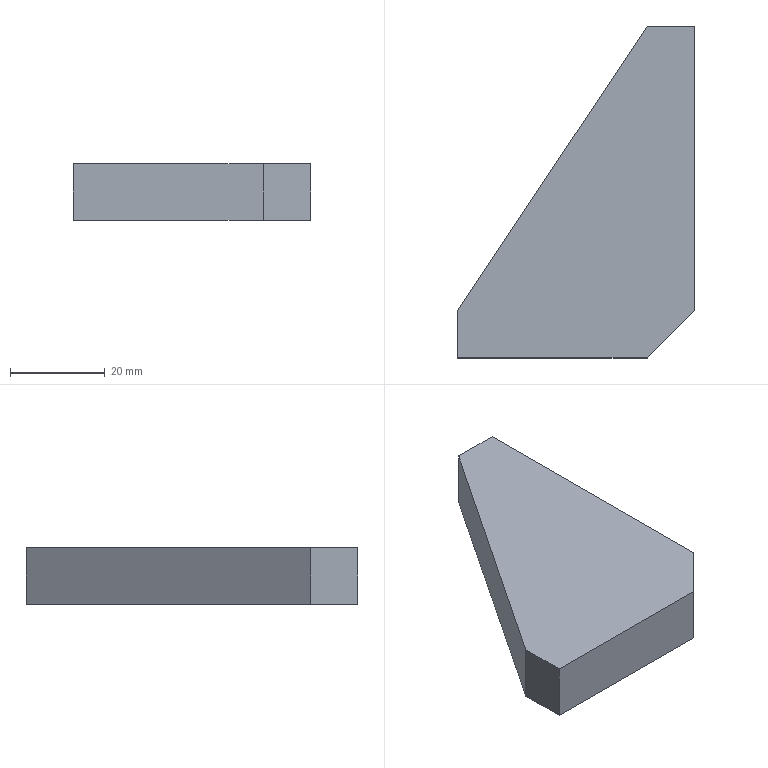Part | STEP file | DCV-000-023 | 1 solid | 8 faces | box 50 x 70 x 12 mm | volume 27000 mm3 | plane 8
STEP:
#1=CARTESIAN_POINT('',(0.,0.,0.));
#2=DIRECTION('',(0.,0.,1.));
#3=DIRECTION('',(1.,0.,0.));
#4=AXIS2_PLACEMENT_3D('',#1,#2,#3);
#5=CARTESIAN_POINT('',(0.,10.,12.));
#6=VERTEX_POINT('',#5);
#7=CARTESIAN_POINT('',(-10.,0.,12.));
#8=VERTEX_POINT('',#7);
#9=CARTESIAN_POINT('',(-2.5,7.5,12.));
#10=DIRECTION('',(-0.7071,-0.7071,0.));
#11=VECTOR('',#10,1.);
#12=LINE('',#9,#11);
#13=CARTESIAN_POINT('',(-25.,35.,12.));
#14=DIRECTION('',(0.,0.,1.));
#15=DIRECTION('',(1.,0.,0.));
#16=AXIS2_PLACEMENT_3D('',#13,#14,#15);
#17=PLANE('',#16);
#18=CARTESIAN_POINT('',(22.5,-27.5));
#19=DIRECTION('',(-0.7071,-0.7071));
#20=VECTOR('',#19,1.);
#21=LINE('',#18,#20);
#22=(GEOMETRIC_REPRESENTATION_CONTEXT(2)PARAMETRIC_REPRESENTATION_CONTEXT()REPRESENTATION_CONTEXT('',''));
#23=DEFINITIONAL_REPRESENTATION('',(#21),#22);
#24=PCURVE('',#17,#23);
#25=CARTESIAN_POINT('',(-5.,5.,0.));
#26=DIRECTION('',(0.7071,-0.7071,0.));
#27=DIRECTION('',(0.,0.,-1.));
#28=AXIS2_PLACEMENT_3D('',#25,#26,#27);
#29=PLANE('',#28);
#30=CARTESIAN_POINT('',(-12.,3.536));
#31=DIRECTION('',(0.,-1.));
#32=VECTOR('',#31,1.);
#33=LINE('',#30,#32);
#34=(GEOMETRIC_REPRESENTATION_CONTEXT(2)PARAMETRIC_REPRESENTATION_CONTEXT()REPRESENTATION_CONTEXT('',''));
#35=DEFINITIONAL_REPRESENTATION('',(#33),#34);
#36=PCURVE('',#29,#35);
#37=SURFACE_CURVE('',#12,(#24,#36),.PCURVE_S1.);
#38=EDGE_CURVE('',#6,#8,#37,.T.);
#39=ORIENTED_EDGE('',*,*,#38,.F.);
#40=CARTESIAN_POINT('',(0.,70.,12.));
#41=VERTEX_POINT('',#40);
#42=CARTESIAN_POINT('',(0.,0.,12.));
#43=DIRECTION('',(0.,1.,0.));
#44=VECTOR('',#43,1.);
#45=LINE('',#42,#44);
#46=CARTESIAN_POINT('',(25.,-35.));
#47=DIRECTION('',(0.,1.));
#48=VECTOR('',#47,1.);
#49=LINE('',#46,#48);
#50=(GEOMETRIC_REPRESENTATION_CONTEXT(2)PARAMETRIC_REPRESENTATION_CONTEXT()REPRESENTATION_CONTEXT('',''));
#51=DEFINITIONAL_REPRESENTATION('',(#49),#50);
#52=PCURVE('',#17,#51);
#53=CARTESIAN_POINT('',(0.,0.,0.));
#54=DIRECTION('',(1.,0.,0.));
#55=DIRECTION('',(0.,1.,0.));
#56=AXIS2_PLACEMENT_3D('',#53,#54,#55);
#57=PLANE('',#56);
#58=CARTESIAN_POINT('',(0.,12.));
#59=DIRECTION('',(1.,0.));
#60=VECTOR('',#59,1.);
#61=LINE('',#58,#60);
#62=(GEOMETRIC_REPRESENTATION_CONTEXT(2)PARAMETRIC_REPRESENTATION_CONTEXT()REPRESENTATION_CONTEXT('',''));
#63=DEFINITIONAL_REPRESENTATION('',(#61),#62);
#64=PCURVE('',#57,#63);
#65=SURFACE_CURVE('',#45,(#52,#64),.PCURVE_S1.);
#66=EDGE_CURVE('',#6,#41,#65,.T.);
#67=ORIENTED_EDGE('',*,*,#66,.T.);
#68=CARTESIAN_POINT('',(-10.,70.,12.));
#69=VERTEX_POINT('',#68);
#70=CARTESIAN_POINT('',(0.,70.,12.));
#71=DIRECTION('',(-1.,0.,0.));
#72=VECTOR('',#71,1.);
#73=LINE('',#70,#72);
#74=CARTESIAN_POINT('',(25.,35.));
#75=DIRECTION('',(-1.,0.));
#76=VECTOR('',#75,1.);
#77=LINE('',#74,#76);
#78=(GEOMETRIC_REPRESENTATION_CONTEXT(2)PARAMETRIC_REPRESENTATION_CONTEXT()REPRESENTATION_CONTEXT('',''));
#79=DEFINITIONAL_REPRESENTATION('',(#77),#78);
#80=PCURVE('',#17,#79);
#81=CARTESIAN_POINT('',(0.,70.,0.));
#82=DIRECTION('',(0.,1.,0.));
#83=DIRECTION('',(1.,0.,0.));
#84=AXIS2_PLACEMENT_3D('',#81,#82,#83);
#85=PLANE('',#84);
#86=CARTESIAN_POINT('',(0.,-12.));
#87=DIRECTION('',(-1.,0.));
#88=VECTOR('',#87,1.);
#89=LINE('',#86,#88);
#90=(GEOMETRIC_REPRESENTATION_CONTEXT(2)PARAMETRIC_REPRESENTATION_CONTEXT()REPRESENTATION_CONTEXT('',''));
#91=DEFINITIONAL_REPRESENTATION('',(#89),#90);
#92=PCURVE('',#85,#91);
#93=SURFACE_CURVE('',#73,(#80,#92),.PCURVE_S1.);
#94=EDGE_CURVE('',#41,#69,#93,.T.);
#95=ORIENTED_EDGE('',*,*,#94,.T.);
#96=CARTESIAN_POINT('',(-50.,10.,12.));
#97=VERTEX_POINT('',#96);
#98=CARTESIAN_POINT('',(-10.,70.,12.));
#99=DIRECTION('',(-0.5547,-0.8321,0.));
#100=VECTOR('',#99,1.);
#101=LINE('',#98,#100);
#102=CARTESIAN_POINT('',(15.,35.));
#103=DIRECTION('',(-0.5547,-0.8321));
#104=VECTOR('',#103,1.);
#105=LINE('',#102,#104);
#106=(GEOMETRIC_REPRESENTATION_CONTEXT(2)PARAMETRIC_REPRESENTATION_CONTEXT()REPRESENTATION_CONTEXT('',''));
#107=DEFINITIONAL_REPRESENTATION('',(#105),#106);
#108=PCURVE('',#17,#107);
#109=CARTESIAN_POINT('',(-10.,70.,0.));
#110=DIRECTION('',(-0.8321,0.5547,0.));
#111=DIRECTION('',(0.,0.,1.));
#112=AXIS2_PLACEMENT_3D('',#109,#110,#111);
#113=PLANE('',#112);
#114=CARTESIAN_POINT('',(12.,0.));
#115=DIRECTION('',(0.,-1.));
#116=VECTOR('',#115,1.);
#117=LINE('',#114,#116);
#118=(GEOMETRIC_REPRESENTATION_CONTEXT(2)PARAMETRIC_REPRESENTATION_CONTEXT()REPRESENTATION_CONTEXT('',''));
#119=DEFINITIONAL_REPRESENTATION('',(#117),#118);
#120=PCURVE('',#113,#119);
#121=SURFACE_CURVE('',#101,(#108,#120),.PCURVE_S1.);
#122=EDGE_CURVE('',#69,#97,#121,.T.);
#123=ORIENTED_EDGE('',*,*,#122,.T.);
#124=CARTESIAN_POINT('',(-50.,0.,12.));
#125=VERTEX_POINT('',#124);
#126=CARTESIAN_POINT('',(-50.,10.,12.));
#127=DIRECTION('',(0.,-1.,0.));
#128=VECTOR('',#127,1.);
#129=LINE('',#126,#128);
#130=CARTESIAN_POINT('',(-25.,-25.));
#131=DIRECTION('',(0.,-1.));
#132=VECTOR('',#131,1.);
#133=LINE('',#130,#132);
#134=(GEOMETRIC_REPRESENTATION_CONTEXT(2)PARAMETRIC_REPRESENTATION_CONTEXT()REPRESENTATION_CONTEXT('',''));
#135=DEFINITIONAL_REPRESENTATION('',(#133),#134);
#136=PCURVE('',#17,#135);
#137=CARTESIAN_POINT('',(-50.,10.,0.));
#138=DIRECTION('',(-1.,0.,0.));
#139=DIRECTION('',(0.,0.,1.));
#140=AXIS2_PLACEMENT_3D('',#137,#138,#139);
#141=PLANE('',#140);
#142=CARTESIAN_POINT('',(12.,0.));
#143=DIRECTION('',(0.,-1.));
#144=VECTOR('',#143,1.);
#145=LINE('',#142,#144);
#146=(GEOMETRIC_REPRESENTATION_CONTEXT(2)PARAMETRIC_REPRESENTATION_CONTEXT()REPRESENTATION_CONTEXT('',''));
#147=DEFINITIONAL_REPRESENTATION('',(#145),#146);
#148=PCURVE('',#141,#147);
#149=SURFACE_CURVE('',#129,(#136,#148),.PCURVE_S1.);
#150=EDGE_CURVE('',#97,#125,#149,.T.);
#151=ORIENTED_EDGE('',*,*,#150,.T.);
#152=CARTESIAN_POINT('',(-50.,0.,12.));
#153=DIRECTION('',(1.,0.,0.));
#154=VECTOR('',#153,1.);
#155=LINE('',#152,#154);
#156=CARTESIAN_POINT('',(-25.,-35.));
#157=DIRECTION('',(1.,0.));
#158=VECTOR('',#157,1.);
#159=LINE('',#156,#158);
#160=(GEOMETRIC_REPRESENTATION_CONTEXT(2)PARAMETRIC_REPRESENTATION_CONTEXT()REPRESENTATION_CONTEXT('',''));
#161=DEFINITIONAL_REPRESENTATION('',(#159),#160);
#162=PCURVE('',#17,#161);
#163=CARTESIAN_POINT('',(-50.,0.,0.));
#164=DIRECTION('',(0.,-1.,0.));
#165=DIRECTION('',(0.,0.,-1.));
#166=AXIS2_PLACEMENT_3D('',#163,#164,#165);
#167=PLANE('',#166);
#168=CARTESIAN_POINT('',(-12.,0.));
#169=DIRECTION('',(0.,1.));
#170=VECTOR('',#169,1.);
#171=LINE('',#168,#170);
#172=(GEOMETRIC_REPRESENTATION_CONTEXT(2)PARAMETRIC_REPRESENTATION_CONTEXT()REPRESENTATION_CONTEXT('',''));
#173=DEFINITIONAL_REPRESENTATION('',(#171),#172);
#174=PCURVE('',#167,#173);
#175=SURFACE_CURVE('',#155,(#162,#174),.PCURVE_S1.);
#176=EDGE_CURVE('',#125,#8,#175,.T.);
#177=ORIENTED_EDGE('',*,*,#176,.T.);
#178=EDGE_LOOP('',(#39,#67,#95,#123,#151,#177));
#179=FACE_BOUND('',#178,.T.);
#180=ADVANCED_FACE('',(#179),#17,.T.);
#181=CARTESIAN_POINT('',(0.,70.,0.));
#182=VERTEX_POINT('',#181);
#183=CARTESIAN_POINT('',(-10.,70.,0.));
#184=VERTEX_POINT('',#183);
#185=CARTESIAN_POINT('',(0.,70.,0.));
#186=DIRECTION('',(-1.,0.,0.));
#187=VECTOR('',#186,1.);
#188=LINE('',#185,#187);
#189=CARTESIAN_POINT('',(0.,0.));
#190=DIRECTION('',(-1.,0.));
#191=VECTOR('',#190,1.);
#192=LINE('',#189,#191);
#193=(GEOMETRIC_REPRESENTATION_CONTEXT(2)PARAMETRIC_REPRESENTATION_CONTEXT()REPRESENTATION_CONTEXT('',''));
#194=DEFINITIONAL_REPRESENTATION('',(#192),#193);
#195=PCURVE('',#85,#194);
#196=CARTESIAN_POINT('',(-25.,35.,0.));
#197=DIRECTION('',(0.,0.,1.));
#198=DIRECTION('',(1.,0.,0.));
#199=AXIS2_PLACEMENT_3D('',#196,#197,#198);
#200=PLANE('',#199);
#201=CARTESIAN_POINT('',(25.,35.));
#202=DIRECTION('',(-1.,0.));
#203=VECTOR('',#202,1.);
#204=LINE('',#201,#203);
#205=(GEOMETRIC_REPRESENTATION_CONTEXT(2)PARAMETRIC_REPRESENTATION_CONTEXT()REPRESENTATION_CONTEXT('',''));
#206=DEFINITIONAL_REPRESENTATION('',(#204),#205);
#207=PCURVE('',#200,#206);
#208=SURFACE_CURVE('',#188,(#195,#207),.PCURVE_S1.);
#209=EDGE_CURVE('',#182,#184,#208,.T.);
#210=ORIENTED_EDGE('',*,*,#209,.T.);
#211=CARTESIAN_POINT('',(-10.,70.,0.));
#212=DIRECTION('',(0.,0.,1.));
#213=VECTOR('',#212,1.);
#214=LINE('',#211,#213);
#215=CARTESIAN_POINT('',(-10.,0.));
#216=DIRECTION('',(0.,-1.));
#217=VECTOR('',#216,1.);
#218=LINE('',#215,#217);
#219=(GEOMETRIC_REPRESENTATION_CONTEXT(2)PARAMETRIC_REPRESENTATION_CONTEXT()REPRESENTATION_CONTEXT('',''));
#220=DEFINITIONAL_REPRESENTATION('',(#218),#219);
#221=PCURVE('',#85,#220);
#222=CARTESIAN_POINT('',(0.,0.));
#223=DIRECTION('',(1.,0.));
#224=VECTOR('',#223,1.);
#225=LINE('',#222,#224);
#226=(GEOMETRIC_REPRESENTATION_CONTEXT(2)PARAMETRIC_REPRESENTATION_CONTEXT()REPRESENTATION_CONTEXT('',''));
#227=DEFINITIONAL_REPRESENTATION('',(#225),#226);
#228=PCURVE('',#113,#227);
#229=SURFACE_CURVE('',#214,(#221,#228),.PCURVE_S1.);
#230=EDGE_CURVE('',#184,#69,#229,.T.);
#231=ORIENTED_EDGE('',*,*,#230,.T.);
#232=ORIENTED_EDGE('',*,*,#94,.F.);
#233=CARTESIAN_POINT('',(0.,70.,0.));
#234=DIRECTION('',(0.,0.,1.));
#235=VECTOR('',#234,1.);
#236=LINE('',#233,#235);
#237=CARTESIAN_POINT('',(0.,0.));
#238=DIRECTION('',(0.,-1.));
#239=VECTOR('',#238,1.);
#240=LINE('',#237,#239);
#241=(GEOMETRIC_REPRESENTATION_CONTEXT(2)PARAMETRIC_REPRESENTATION_CONTEXT()REPRESENTATION_CONTEXT('',''));
#242=DEFINITIONAL_REPRESENTATION('',(#240),#241);
#243=PCURVE('',#85,#242);
#244=CARTESIAN_POINT('',(70.,0.));
#245=DIRECTION('',(0.,1.));
#246=VECTOR('',#245,1.);
#247=LINE('',#244,#246);
#248=(GEOMETRIC_REPRESENTATION_CONTEXT(2)PARAMETRIC_REPRESENTATION_CONTEXT()REPRESENTATION_CONTEXT('',''));
#249=DEFINITIONAL_REPRESENTATION('',(#247),#248);
#250=PCURVE('',#57,#249);
#251=SURFACE_CURVE('',#236,(#243,#250),.PCURVE_S1.);
#252=EDGE_CURVE('',#182,#41,#251,.T.);
#253=ORIENTED_EDGE('',*,*,#252,.F.);
#254=EDGE_LOOP('',(#210,#231,#232,#253));
#255=FACE_BOUND('',#254,.T.);
#256=ADVANCED_FACE('',(#255),#85,.T.);
#257=CARTESIAN_POINT('',(-50.,10.,0.));
#258=VERTEX_POINT('',#257);
#259=CARTESIAN_POINT('',(-10.,70.,0.));
#260=DIRECTION('',(-0.5547,-0.8321,0.));
#261=VECTOR('',#260,1.);
#262=LINE('',#259,#261);
#263=CARTESIAN_POINT('',(0.,0.));
#264=DIRECTION('',(0.,-1.));
#265=VECTOR('',#264,1.);
#266=LINE('',#263,#265);
#267=(GEOMETRIC_REPRESENTATION_CONTEXT(2)PARAMETRIC_REPRESENTATION_CONTEXT()REPRESENTATION_CONTEXT('',''));
#268=DEFINITIONAL_REPRESENTATION('',(#266),#267);
#269=PCURVE('',#113,#268);
#270=CARTESIAN_POINT('',(15.,35.));
#271=DIRECTION('',(-0.5547,-0.8321));
#272=VECTOR('',#271,1.);
#273=LINE('',#270,#272);
#274=(GEOMETRIC_REPRESENTATION_CONTEXT(2)PARAMETRIC_REPRESENTATION_CONTEXT()REPRESENTATION_CONTEXT('',''));
#275=DEFINITIONAL_REPRESENTATION('',(#273),#274);
#276=PCURVE('',#200,#275);
#277=SURFACE_CURVE('',#262,(#269,#276),.PCURVE_S1.);
#278=EDGE_CURVE('',#184,#258,#277,.T.);
#279=ORIENTED_EDGE('',*,*,#278,.T.);
#280=CARTESIAN_POINT('',(-50.,10.,0.));
#281=DIRECTION('',(0.,0.,1.));
#282=VECTOR('',#281,1.);
#283=LINE('',#280,#282);
#284=CARTESIAN_POINT('',(0.,-72.111));
#285=DIRECTION('',(1.,0.));
#286=VECTOR('',#285,1.);
#287=LINE('',#284,#286);
#288=(GEOMETRIC_REPRESENTATION_CONTEXT(2)PARAMETRIC_REPRESENTATION_CONTEXT()REPRESENTATION_CONTEXT('',''));
#289=DEFINITIONAL_REPRESENTATION('',(#287),#288);
#290=PCURVE('',#113,#289);
#291=CARTESIAN_POINT('',(0.,0.));
#292=DIRECTION('',(1.,0.));
#293=VECTOR('',#292,1.);
#294=LINE('',#291,#293);
#295=(GEOMETRIC_REPRESENTATION_CONTEXT(2)PARAMETRIC_REPRESENTATION_CONTEXT()REPRESENTATION_CONTEXT('',''));
#296=DEFINITIONAL_REPRESENTATION('',(#294),#295);
#297=PCURVE('',#141,#296);
#298=SURFACE_CURVE('',#283,(#290,#297),.PCURVE_S1.);
#299=EDGE_CURVE('',#258,#97,#298,.T.);
#300=ORIENTED_EDGE('',*,*,#299,.T.);
#301=ORIENTED_EDGE('',*,*,#122,.F.);
#302=ORIENTED_EDGE('',*,*,#230,.F.);
#303=EDGE_LOOP('',(#279,#300,#301,#302));
#304=FACE_BOUND('',#303,.T.);
#305=ADVANCED_FACE('',(#304),#113,.T.);
#306=CARTESIAN_POINT('',(-50.,0.,0.));
#307=VERTEX_POINT('',#306);
#308=CARTESIAN_POINT('',(-50.,10.,0.));
#309=DIRECTION('',(0.,-1.,0.));
#310=VECTOR('',#309,1.);
#311=LINE('',#308,#310);
#312=CARTESIAN_POINT('',(0.,0.));
#313=DIRECTION('',(0.,-1.));
#314=VECTOR('',#313,1.);
#315=LINE('',#312,#314);
#316=(GEOMETRIC_REPRESENTATION_CONTEXT(2)PARAMETRIC_REPRESENTATION_CONTEXT()REPRESENTATION_CONTEXT('',''));
#317=DEFINITIONAL_REPRESENTATION('',(#315),#316);
#318=PCURVE('',#141,#317);
#319=CARTESIAN_POINT('',(-25.,-25.));
#320=DIRECTION('',(0.,-1.));
#321=VECTOR('',#320,1.);
#322=LINE('',#319,#321);
#323=(GEOMETRIC_REPRESENTATION_CONTEXT(2)PARAMETRIC_REPRESENTATION_CONTEXT()REPRESENTATION_CONTEXT('',''));
#324=DEFINITIONAL_REPRESENTATION('',(#322),#323);
#325=PCURVE('',#200,#324);
#326=SURFACE_CURVE('',#311,(#318,#325),.PCURVE_S1.);
#327=EDGE_CURVE('',#258,#307,#326,.T.);
#328=ORIENTED_EDGE('',*,*,#327,.T.);
#329=CARTESIAN_POINT('',(-50.,0.,0.));
#330=DIRECTION('',(0.,0.,1.));
#331=VECTOR('',#330,1.);
#332=LINE('',#329,#331);
#333=CARTESIAN_POINT('',(0.,-10.));
#334=DIRECTION('',(1.,0.));
#335=VECTOR('',#334,1.);
#336=LINE('',#333,#335);
#337=(GEOMETRIC_REPRESENTATION_CONTEXT(2)PARAMETRIC_REPRESENTATION_CONTEXT()REPRESENTATION_CONTEXT('',''));
#338=DEFINITIONAL_REPRESENTATION('',(#336),#337);
#339=PCURVE('',#141,#338);
#340=CARTESIAN_POINT('',(0.,0.));
#341=DIRECTION('',(-1.,0.));
#342=VECTOR('',#341,1.);
#343=LINE('',#340,#342);
#344=(GEOMETRIC_REPRESENTATION_CONTEXT(2)PARAMETRIC_REPRESENTATION_CONTEXT()REPRESENTATION_CONTEXT('',''));
#345=DEFINITIONAL_REPRESENTATION('',(#343),#344);
#346=PCURVE('',#167,#345);
#347=SURFACE_CURVE('',#332,(#339,#346),.PCURVE_S1.);
#348=EDGE_CURVE('',#307,#125,#347,.T.);
#349=ORIENTED_EDGE('',*,*,#348,.T.);
#350=ORIENTED_EDGE('',*,*,#150,.F.);
#351=ORIENTED_EDGE('',*,*,#299,.F.);
#352=EDGE_LOOP('',(#328,#349,#350,#351));
#353=FACE_BOUND('',#352,.T.);
#354=ADVANCED_FACE('',(#353),#141,.T.);
#355=CARTESIAN_POINT('',(0.,10.,0.));
#356=VERTEX_POINT('',#355);
#357=CARTESIAN_POINT('',(0.,10.,0.));
#358=DIRECTION('',(0.,0.,1.));
#359=VECTOR('',#358,1.);
#360=LINE('',#357,#359);
#361=CARTESIAN_POINT('',(10.,0.));
#362=DIRECTION('',(0.,1.));
#363=VECTOR('',#362,1.);
#364=LINE('',#361,#363);
#365=(GEOMETRIC_REPRESENTATION_CONTEXT(2)PARAMETRIC_REPRESENTATION_CONTEXT()REPRESENTATION_CONTEXT('',''));
#366=DEFINITIONAL_REPRESENTATION('',(#364),#365);
#367=PCURVE('',#57,#366);
#368=CARTESIAN_POINT('',(0.,7.071));
#369=DIRECTION('',(-1.,0.));
#370=VECTOR('',#369,1.);
#371=LINE('',#368,#370);
#372=(GEOMETRIC_REPRESENTATION_CONTEXT(2)PARAMETRIC_REPRESENTATION_CONTEXT()REPRESENTATION_CONTEXT('',''));
#373=DEFINITIONAL_REPRESENTATION('',(#371),#372);
#374=PCURVE('',#29,#373);
#375=SURFACE_CURVE('',#360,(#367,#374),.PCURVE_S1.);
#376=EDGE_CURVE('',#356,#6,#375,.T.);
#377=ORIENTED_EDGE('',*,*,#376,.F.);
#378=CARTESIAN_POINT('',(0.,0.,0.));
#379=DIRECTION('',(0.,1.,0.));
#380=VECTOR('',#379,1.);
#381=LINE('',#378,#380);
#382=CARTESIAN_POINT('',(0.,0.));
#383=DIRECTION('',(1.,0.));
#384=VECTOR('',#383,1.);
#385=LINE('',#382,#384);
#386=(GEOMETRIC_REPRESENTATION_CONTEXT(2)PARAMETRIC_REPRESENTATION_CONTEXT()REPRESENTATION_CONTEXT('',''));
#387=DEFINITIONAL_REPRESENTATION('',(#385),#386);
#388=PCURVE('',#57,#387);
#389=CARTESIAN_POINT('',(25.,-35.));
#390=DIRECTION('',(0.,1.));
#391=VECTOR('',#390,1.);
#392=LINE('',#389,#391);
#393=(GEOMETRIC_REPRESENTATION_CONTEXT(2)PARAMETRIC_REPRESENTATION_CONTEXT()REPRESENTATION_CONTEXT('',''));
#394=DEFINITIONAL_REPRESENTATION('',(#392),#393);
#395=PCURVE('',#200,#394);
#396=SURFACE_CURVE('',#381,(#388,#395),.PCURVE_S1.);
#397=EDGE_CURVE('',#356,#182,#396,.T.);
#398=ORIENTED_EDGE('',*,*,#397,.T.);
#399=ORIENTED_EDGE('',*,*,#252,.T.);
#400=ORIENTED_EDGE('',*,*,#66,.F.);
#401=EDGE_LOOP('',(#377,#398,#399,#400));
#402=FACE_BOUND('',#401,.T.);
#403=ADVANCED_FACE('',(#402),#57,.T.);
#404=CARTESIAN_POINT('',(-10.,0.,0.));
#405=VERTEX_POINT('',#404);
#406=CARTESIAN_POINT('',(-10.,0.,0.));
#407=DIRECTION('',(0.,0.,-1.));
#408=VECTOR('',#407,1.);
#409=LINE('',#406,#408);
#410=CARTESIAN_POINT('',(0.,40.));
#411=DIRECTION('',(1.,0.));
#412=VECTOR('',#411,1.);
#413=LINE('',#410,#412);
#414=(GEOMETRIC_REPRESENTATION_CONTEXT(2)PARAMETRIC_REPRESENTATION_CONTEXT()REPRESENTATION_CONTEXT('',''));
#415=DEFINITIONAL_REPRESENTATION('',(#413),#414);
#416=PCURVE('',#167,#415);
#417=CARTESIAN_POINT('',(0.,-7.071));
#418=DIRECTION('',(1.,0.));
#419=VECTOR('',#418,1.);
#420=LINE('',#417,#419);
#421=(GEOMETRIC_REPRESENTATION_CONTEXT(2)PARAMETRIC_REPRESENTATION_CONTEXT()REPRESENTATION_CONTEXT('',''));
#422=DEFINITIONAL_REPRESENTATION('',(#420),#421);
#423=PCURVE('',#29,#422);
#424=SURFACE_CURVE('',#409,(#416,#423),.PCURVE_S1.);
#425=EDGE_CURVE('',#8,#405,#424,.T.);
#426=ORIENTED_EDGE('',*,*,#425,.F.);
#427=ORIENTED_EDGE('',*,*,#176,.F.);
#428=ORIENTED_EDGE('',*,*,#348,.F.);
#429=CARTESIAN_POINT('',(-50.,0.,0.));
#430=DIRECTION('',(1.,0.,0.));
#431=VECTOR('',#430,1.);
#432=LINE('',#429,#431);
#433=CARTESIAN_POINT('',(0.,0.));
#434=DIRECTION('',(0.,1.));
#435=VECTOR('',#434,1.);
#436=LINE('',#433,#435);
#437=(GEOMETRIC_REPRESENTATION_CONTEXT(2)PARAMETRIC_REPRESENTATION_CONTEXT()REPRESENTATION_CONTEXT('',''));
#438=DEFINITIONAL_REPRESENTATION('',(#436),#437);
#439=PCURVE('',#167,#438);
#440=CARTESIAN_POINT('',(-25.,-35.));
#441=DIRECTION('',(1.,0.));
#442=VECTOR('',#441,1.);
#443=LINE('',#440,#442);
#444=(GEOMETRIC_REPRESENTATION_CONTEXT(2)PARAMETRIC_REPRESENTATION_CONTEXT()REPRESENTATION_CONTEXT('',''));
#445=DEFINITIONAL_REPRESENTATION('',(#443),#444);
#446=PCURVE('',#200,#445);
#447=SURFACE_CURVE('',#432,(#439,#446),.PCURVE_S1.);
#448=EDGE_CURVE('',#307,#405,#447,.T.);
#449=ORIENTED_EDGE('',*,*,#448,.T.);
#450=EDGE_LOOP('',(#426,#427,#428,#449));
#451=FACE_BOUND('',#450,.T.);
#452=ADVANCED_FACE('',(#451),#167,.T.);
#453=CARTESIAN_POINT('',(-2.5,7.5,0.));
#454=DIRECTION('',(0.7071,0.7071,0.));
#455=VECTOR('',#454,1.);
#456=LINE('',#453,#455);
#457=CARTESIAN_POINT('',(22.5,-27.5));
#458=DIRECTION('',(0.7071,0.7071));
#459=VECTOR('',#458,1.);
#460=LINE('',#457,#459);
#461=(GEOMETRIC_REPRESENTATION_CONTEXT(2)PARAMETRIC_REPRESENTATION_CONTEXT()REPRESENTATION_CONTEXT('',''));
#462=DEFINITIONAL_REPRESENTATION('',(#460),#461);
#463=PCURVE('',#200,#462);
#464=CARTESIAN_POINT('',(0.,3.536));
#465=DIRECTION('',(0.,1.));
#466=VECTOR('',#465,1.);
#467=LINE('',#464,#466);
#468=(GEOMETRIC_REPRESENTATION_CONTEXT(2)PARAMETRIC_REPRESENTATION_CONTEXT()REPRESENTATION_CONTEXT('',''));
#469=DEFINITIONAL_REPRESENTATION('',(#467),#468);
#470=PCURVE('',#29,#469);
#471=SURFACE_CURVE('',#456,(#463,#470),.PCURVE_S1.);
#472=EDGE_CURVE('',#405,#356,#471,.T.);
#473=ORIENTED_EDGE('',*,*,#472,.F.);
#474=ORIENTED_EDGE('',*,*,#448,.F.);
#475=ORIENTED_EDGE('',*,*,#327,.F.);
#476=ORIENTED_EDGE('',*,*,#278,.F.);
#477=ORIENTED_EDGE('',*,*,#209,.F.);
#478=ORIENTED_EDGE('',*,*,#397,.F.);
#479=EDGE_LOOP('',(#473,#474,#475,#476,#477,#478));
#480=FACE_BOUND('',#479,.T.);
#481=ADVANCED_FACE('',(#480),#200,.F.);
#482=ORIENTED_EDGE('',*,*,#38,.T.);
#483=ORIENTED_EDGE('',*,*,#425,.T.);
#484=ORIENTED_EDGE('',*,*,#472,.T.);
#485=ORIENTED_EDGE('',*,*,#376,.T.);
#486=EDGE_LOOP('',(#482,#483,#484,#485));
#487=FACE_BOUND('',#486,.T.);
#488=ADVANCED_FACE('',(#487),#29,.T.);
#489=CLOSED_SHELL('',(#180,#256,#305,#354,#403,#452,#481,#488));
#490=MANIFOLD_SOLID_BREP('',#489);
#491=(LENGTH_UNIT()NAMED_UNIT(*)SI_UNIT(.MILLI.,.METRE.));
#492=UNCERTAINTY_MEASURE_WITH_UNIT(LENGTH_MEASURE(0.0000001),#491,'','');
#493=(NAMED_UNIT(*)PLANE_ANGLE_UNIT()SI_UNIT($,.RADIAN.));
#494=(NAMED_UNIT(*)SI_UNIT($,.STERADIAN.)SOLID_ANGLE_UNIT());
#495=(GEOMETRIC_REPRESENTATION_CONTEXT(3)GLOBAL_UNCERTAINTY_ASSIGNED_CONTEXT((#492))GLOBAL_UNIT_ASSIGNED_CONTEXT((#491,#493,#494))REPRESENTATION_CONTEXT('',''));
#496=ADVANCED_BREP_SHAPE_REPRESENTATION('',(#4,#490),#495);